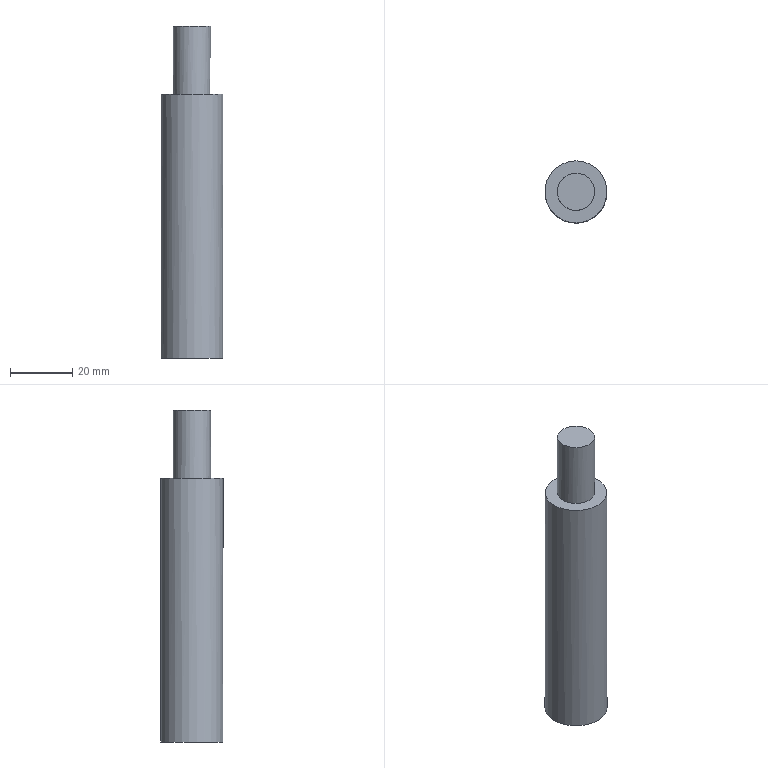Part | NX | features solid 2 | 1 solid | 5 faces | box 20 x 20 x 107 mm | volume 29192 mm3 | plane 3 | cylinder 2 | commonest cylinder face diameters 12 x1 20 x1
STEP:
#1=CARTESIAN_POINT('',(392.,-99.,-5.));
#2=VERTEX_POINT('',#1);
#3=CARTESIAN_POINT('',(392.,-109.,-5.));
#4=DIRECTION('',(0.,0.,-1.));
#5=DIRECTION('',(0.,1.,0.));
#6=AXIS2_PLACEMENT_3D('',#3,#4,#5);
#7=CIRCLE('',#6,10.);
#8=EDGE_CURVE('',#2,#2,#7,.T.);
#9=ORIENTED_EDGE('',*,*,#8,.F.);
#10=EDGE_LOOP('',(#9));
#11=FACE_BOUND('',#10,.T.);
#12=CARTESIAN_POINT('',(392.,-103.,-5.));
#13=VERTEX_POINT('',#12);
#14=CARTESIAN_POINT('',(392.,-109.,-5.));
#15=DIRECTION('',(0.,0.,-1.));
#16=DIRECTION('',(0.,1.,0.));
#17=AXIS2_PLACEMENT_3D('',#14,#15,#16);
#18=CIRCLE('',#17,6.);
#19=EDGE_CURVE('',#13,#13,#18,.F.);
#20=ORIENTED_EDGE('',*,*,#19,.F.);
#21=EDGE_LOOP('',(#20));
#22=FACE_BOUND('',#21,.T.);
#23=CARTESIAN_POINT('',(212.,-170.,-5.));
#24=DIRECTION('',(0.,0.,-1.));
#25=DIRECTION('',(0.,1.,0.));
#26=AXIS2_PLACEMENT_3D('',#23,#24,#25);
#27=PLANE('',#26);
#28=ADVANCED_FACE('',(#11,#22),#27,.F.);
#29=CARTESIAN_POINT('',(402.,-109.,-90.));
#30=VERTEX_POINT('',#29);
#31=CARTESIAN_POINT('',(392.,-109.,-90.));
#32=DIRECTION('',(0.,0.,1.));
#33=DIRECTION('',(1.,0.,0.));
#34=AXIS2_PLACEMENT_3D('',#31,#32,#33);
#35=CIRCLE('',#34,10.);
#36=EDGE_CURVE('',#30,#30,#35,.T.);
#37=ORIENTED_EDGE('',*,*,#36,.F.);
#38=EDGE_LOOP('',(#37));
#39=FACE_BOUND('',#38,.T.);
#40=CARTESIAN_POINT('',(392.,-109.,-90.));
#41=DIRECTION('',(0.,0.,1.));
#42=DIRECTION('',(1.,0.,0.));
#43=AXIS2_PLACEMENT_3D('',#40,#41,#42);
#44=PLANE('',#43);
#45=ADVANCED_FACE('',(#39),#44,.F.);
#46=ORIENTED_EDGE('',*,*,#8,.T.);
#47=EDGE_LOOP('',(#46));
#48=FACE_BOUND('',#47,.T.);
#49=ORIENTED_EDGE('',*,*,#36,.T.);
#50=EDGE_LOOP('',(#49));
#51=FACE_BOUND('',#50,.T.);
#52=CARTESIAN_POINT('',(392.,-109.,70.));
#53=DIRECTION('',(0.,0.,-1.));
#54=DIRECTION('',(-1.,0.,0.));
#55=AXIS2_PLACEMENT_3D('',#52,#53,#54);
#56=CYLINDRICAL_SURFACE('',#55,10.);
#57=ADVANCED_FACE('',(#48,#51),#56,.T.);
#58=CARTESIAN_POINT('',(398.,-109.,17.));
#59=VERTEX_POINT('',#58);
#60=CARTESIAN_POINT('',(392.,-109.,17.));
#61=DIRECTION('',(0.,0.,1.));
#62=DIRECTION('',(1.,0.,0.));
#63=AXIS2_PLACEMENT_3D('',#60,#61,#62);
#64=CIRCLE('',#63,6.);
#65=EDGE_CURVE('',#59,#59,#64,.T.);
#66=ORIENTED_EDGE('',*,*,#65,.F.);
#67=EDGE_LOOP('',(#66));
#68=FACE_BOUND('',#67,.T.);
#69=ORIENTED_EDGE('',*,*,#19,.T.);
#70=EDGE_LOOP('',(#69));
#71=FACE_BOUND('',#70,.T.);
#72=CARTESIAN_POINT('',(392.,-109.,70.));
#73=DIRECTION('',(0.,0.,-1.));
#74=DIRECTION('',(-1.,0.,0.));
#75=AXIS2_PLACEMENT_3D('',#72,#73,#74);
#76=CYLINDRICAL_SURFACE('',#75,6.);
#77=ADVANCED_FACE('',(#68,#71),#76,.T.);
#78=ORIENTED_EDGE('',*,*,#65,.T.);
#79=EDGE_LOOP('',(#78));
#80=FACE_BOUND('',#79,.T.);
#81=CARTESIAN_POINT('',(335.,-115.,17.));
#82=DIRECTION('',(0.,0.,1.));
#83=DIRECTION('',(-1.,0.,0.));
#84=AXIS2_PLACEMENT_3D('',#81,#82,#83);
#85=PLANE('',#84);
#86=ADVANCED_FACE('',(#80),#85,.T.);
#87=CLOSED_SHELL('',(#28,#45,#57,#77,#86));
#88=MANIFOLD_SOLID_BREP('',#87);
#89=(LENGTH_UNIT()NAMED_UNIT(*)SI_UNIT(.MILLI.,.METRE.));
#90=UNCERTAINTY_MEASURE_WITH_UNIT(LENGTH_MEASURE(0.00001),#89,'','');
#91=(NAMED_UNIT(*)PLANE_ANGLE_UNIT()SI_UNIT($,.RADIAN.));
#92=(NAMED_UNIT(*)SI_UNIT($,.STERADIAN.)SOLID_ANGLE_UNIT());
#93=(GEOMETRIC_REPRESENTATION_CONTEXT(3)GLOBAL_UNCERTAINTY_ASSIGNED_CONTEXT((#90))GLOBAL_UNIT_ASSIGNED_CONTEXT((#89,#91,#92))REPRESENTATION_CONTEXT('',''));
#94=ADVANCED_BREP_SHAPE_REPRESENTATION('',(#88),#93);